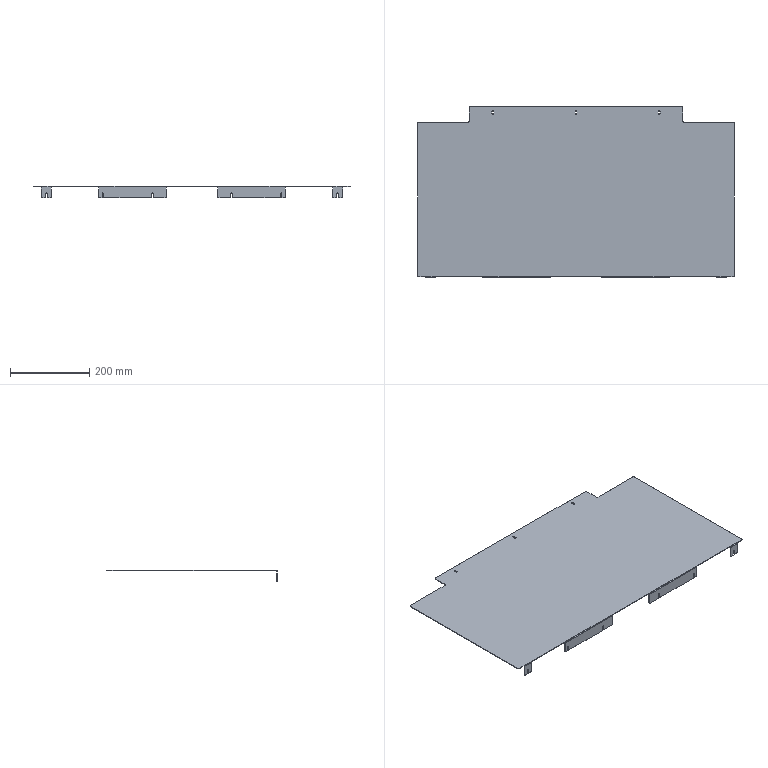Part | STEP file | Line stopper plate | 1 solid | 94 faces | box 800 x 431 x 30 mm | volume 516055 mm3 | plane 58 | cylinder 36 | commonest cylinder face diameters 6 x16 4.3 x6 4.5 x6 1 x4 4 x4